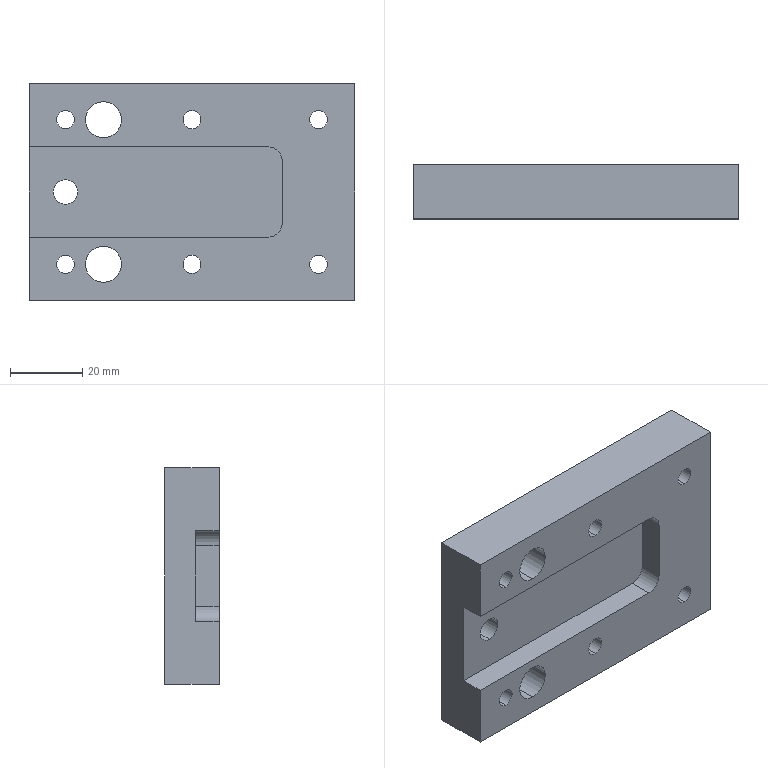Part | STEP file | Ngam kep 9 | 1 solid | 30 faces | box 90 x 15 x 60 mm | volume 65238 mm3 | cylinder 20 | plane 10 | commonest cylinder face diameters 5 x12 10 x4 6.8 x2 8 x2